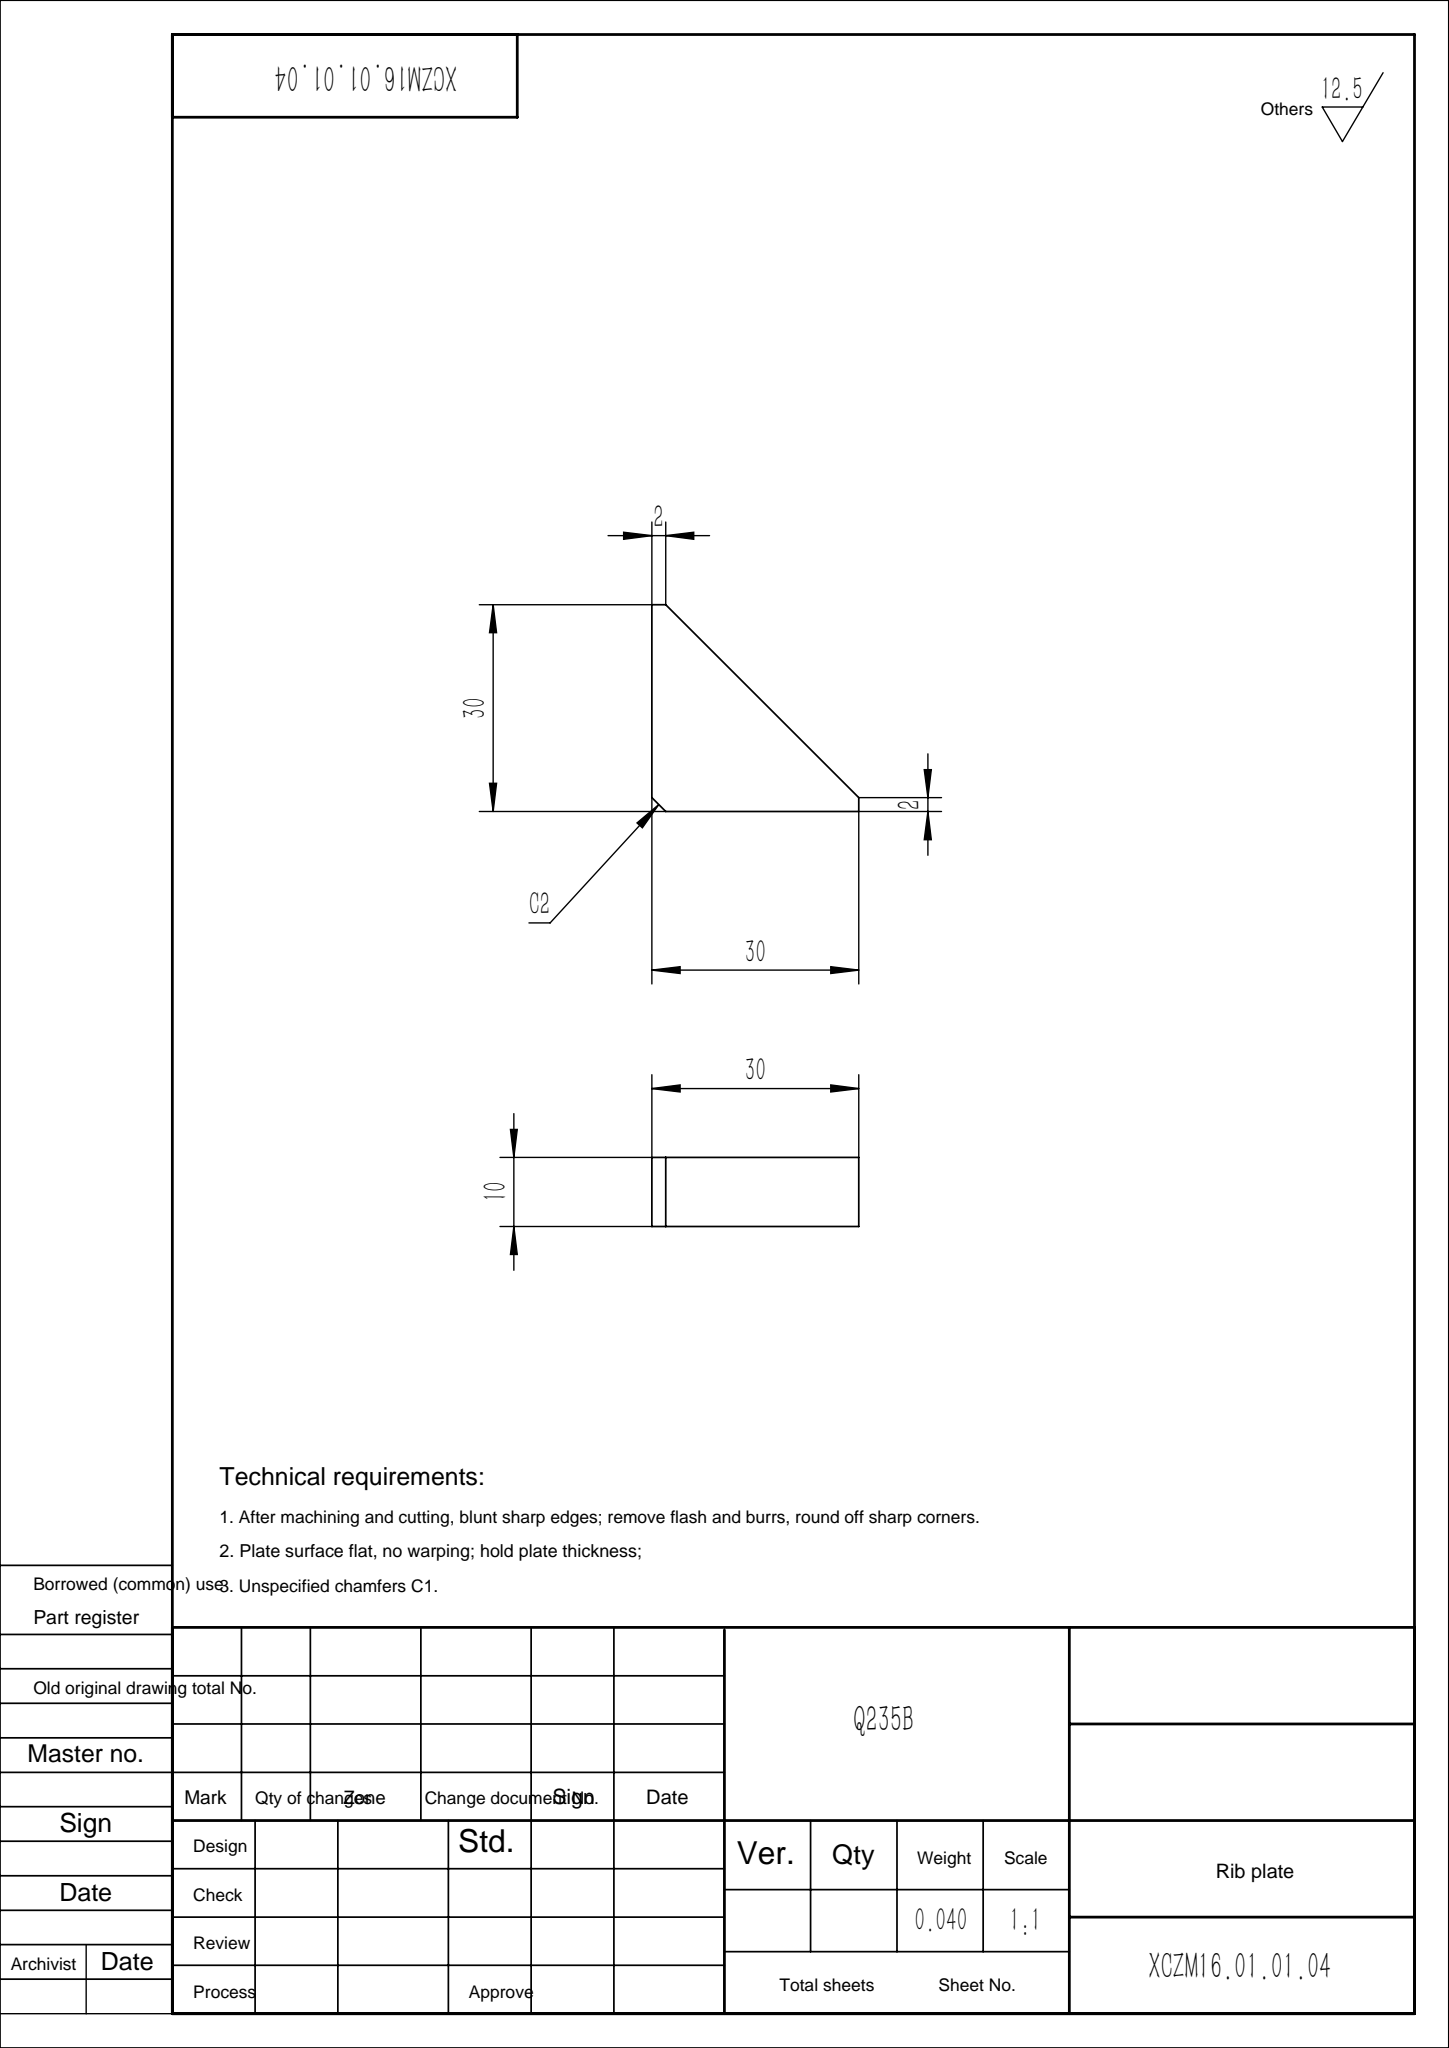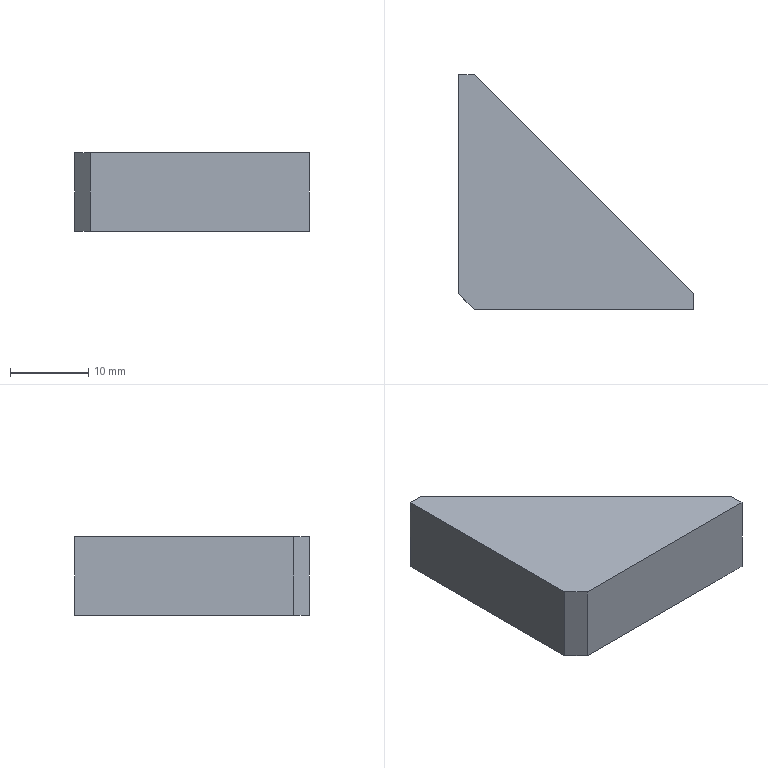Part | SolidWorks | features Chamfer 1, Extrusion 1 | 1 solid | 8 faces | box 30 x 30 x 10 mm | volume 5060 mm3 | plane 8
STEP:
#1=CARTESIAN_POINT('',(2.,30.,0.));
#2=VERTEX_POINT('',#1);
#3=CARTESIAN_POINT('',(0.,30.,0.));
#4=VERTEX_POINT('',#3);
#5=CARTESIAN_POINT('',(2.,30.,0.));
#6=DIRECTION('',(-1.,0.,0.));
#7=VECTOR('',#6,1000.);
#8=LINE('',#5,#7);
#9=EDGE_CURVE('',#2,#4,#8,.T.);
#10=ORIENTED_EDGE('',*,*,#9,.T.);
#11=CARTESIAN_POINT('',(0.,30.,10.));
#12=VERTEX_POINT('',#11);
#13=CARTESIAN_POINT('',(0.,30.,10.));
#14=DIRECTION('',(0.,0.,-1.));
#15=VECTOR('',#14,1000.);
#16=LINE('',#13,#15);
#17=EDGE_CURVE('',#12,#4,#16,.T.);
#18=ORIENTED_EDGE('',*,*,#17,.F.);
#19=CARTESIAN_POINT('',(2.,30.,10.));
#20=VERTEX_POINT('',#19);
#21=CARTESIAN_POINT('',(2.,30.,10.));
#22=DIRECTION('',(-1.,0.,0.));
#23=VECTOR('',#22,1000.);
#24=LINE('',#21,#23);
#25=EDGE_CURVE('',#20,#12,#24,.T.);
#26=ORIENTED_EDGE('',*,*,#25,.F.);
#27=CARTESIAN_POINT('',(2.,30.,10.));
#28=DIRECTION('',(0.,0.,-1.));
#29=VECTOR('',#28,1000.);
#30=LINE('',#27,#29);
#31=EDGE_CURVE('',#20,#2,#30,.T.);
#32=ORIENTED_EDGE('',*,*,#31,.T.);
#33=EDGE_LOOP('',(#10,#18,#26,#32));
#34=FACE_OUTER_BOUND('',#33,.T.);
#35=CARTESIAN_POINT('',(2.,30.,10.));
#36=DIRECTION('',(0.,-1.,0.));
#37=DIRECTION('',(0.,0.,-1.));
#38=AXIS2_PLACEMENT_3D('',#35,#36,#37);
#39=PLANE('',#38);
#40=ADVANCED_FACE('',(#34),#39,.F.);
#41=CARTESIAN_POINT('',(0.,2.,0.));
#42=VERTEX_POINT('',#41);
#43=CARTESIAN_POINT('',(0.,30.,0.));
#44=DIRECTION('',(0.,-1.,0.));
#45=VECTOR('',#44,1000.);
#46=LINE('',#43,#45);
#47=EDGE_CURVE('',#4,#42,#46,.T.);
#48=ORIENTED_EDGE('',*,*,#47,.T.);
#49=CARTESIAN_POINT('',(0.,2.,10.));
#50=VERTEX_POINT('',#49);
#51=CARTESIAN_POINT('',(0.,2.,10.));
#52=DIRECTION('',(0.,0.,1.));
#53=VECTOR('',#52,1000.);
#54=LINE('',#51,#53);
#55=EDGE_CURVE('',#42,#50,#54,.T.);
#56=ORIENTED_EDGE('',*,*,#55,.T.);
#57=CARTESIAN_POINT('',(0.,30.,10.));
#58=DIRECTION('',(0.,-1.,0.));
#59=VECTOR('',#58,1000.);
#60=LINE('',#57,#59);
#61=EDGE_CURVE('',#12,#50,#60,.T.);
#62=ORIENTED_EDGE('',*,*,#61,.F.);
#63=ORIENTED_EDGE('',*,*,#17,.T.);
#64=EDGE_LOOP('',(#48,#56,#62,#63));
#65=FACE_OUTER_BOUND('',#64,.T.);
#66=CARTESIAN_POINT('',(0.,30.,10.));
#67=DIRECTION('',(1.,0.,0.));
#68=DIRECTION('',(0.,1.,0.));
#69=AXIS2_PLACEMENT_3D('',#66,#67,#68);
#70=PLANE('',#69);
#71=ADVANCED_FACE('',(#65),#70,.F.);
#72=CARTESIAN_POINT('',(2.,0.,10.));
#73=VERTEX_POINT('',#72);
#74=CARTESIAN_POINT('',(30.,0.,10.));
#75=VERTEX_POINT('',#74);
#76=CARTESIAN_POINT('',(0.,0.,10.));
#77=DIRECTION('',(1.,0.,0.));
#78=VECTOR('',#77,1000.);
#79=LINE('',#76,#78);
#80=EDGE_CURVE('',#73,#75,#79,.T.);
#81=ORIENTED_EDGE('',*,*,#80,.F.);
#82=CARTESIAN_POINT('',(2.,0.,0.));
#83=VERTEX_POINT('',#82);
#84=CARTESIAN_POINT('',(2.,0.,10.));
#85=DIRECTION('',(0.,0.,-1.));
#86=VECTOR('',#85,1000.);
#87=LINE('',#84,#86);
#88=EDGE_CURVE('',#73,#83,#87,.T.);
#89=ORIENTED_EDGE('',*,*,#88,.T.);
#90=CARTESIAN_POINT('',(30.,0.,0.));
#91=VERTEX_POINT('',#90);
#92=CARTESIAN_POINT('',(0.,0.,0.));
#93=DIRECTION('',(1.,0.,0.));
#94=VECTOR('',#93,1000.);
#95=LINE('',#92,#94);
#96=EDGE_CURVE('',#83,#91,#95,.T.);
#97=ORIENTED_EDGE('',*,*,#96,.T.);
#98=CARTESIAN_POINT('',(30.,0.,10.));
#99=DIRECTION('',(0.,0.,-1.));
#100=VECTOR('',#99,1000.);
#101=LINE('',#98,#100);
#102=EDGE_CURVE('',#75,#91,#101,.T.);
#103=ORIENTED_EDGE('',*,*,#102,.F.);
#104=EDGE_LOOP('',(#81,#89,#97,#103));
#105=FACE_OUTER_BOUND('',#104,.T.);
#106=CARTESIAN_POINT('',(0.,0.,10.));
#107=DIRECTION('',(0.,1.,0.));
#108=DIRECTION('',(0.,0.,1.));
#109=AXIS2_PLACEMENT_3D('',#106,#107,#108);
#110=PLANE('',#109);
#111=ADVANCED_FACE('',(#105),#110,.F.);
#112=CARTESIAN_POINT('',(30.,2.,0.));
#113=VERTEX_POINT('',#112);
#114=CARTESIAN_POINT('',(30.,0.,0.));
#115=DIRECTION('',(0.,1.,0.));
#116=VECTOR('',#115,1000.);
#117=LINE('',#114,#116);
#118=EDGE_CURVE('',#91,#113,#117,.T.);
#119=ORIENTED_EDGE('',*,*,#118,.T.);
#120=CARTESIAN_POINT('',(30.,2.,10.));
#121=VERTEX_POINT('',#120);
#122=CARTESIAN_POINT('',(30.,2.,10.));
#123=DIRECTION('',(0.,0.,-1.));
#124=VECTOR('',#123,1000.);
#125=LINE('',#122,#124);
#126=EDGE_CURVE('',#121,#113,#125,.T.);
#127=ORIENTED_EDGE('',*,*,#126,.F.);
#128=CARTESIAN_POINT('',(30.,0.,10.));
#129=DIRECTION('',(0.,1.,0.));
#130=VECTOR('',#129,1000.);
#131=LINE('',#128,#130);
#132=EDGE_CURVE('',#75,#121,#131,.T.);
#133=ORIENTED_EDGE('',*,*,#132,.F.);
#134=ORIENTED_EDGE('',*,*,#102,.T.);
#135=EDGE_LOOP('',(#119,#127,#133,#134));
#136=FACE_OUTER_BOUND('',#135,.T.);
#137=CARTESIAN_POINT('',(30.,0.,10.));
#138=DIRECTION('',(-1.,0.,0.));
#139=DIRECTION('',(0.,0.,1.));
#140=AXIS2_PLACEMENT_3D('',#137,#138,#139);
#141=PLANE('',#140);
#142=ADVANCED_FACE('',(#136),#141,.F.);
#143=CARTESIAN_POINT('',(30.,2.,0.));
#144=DIRECTION('',(-0.7071,0.7071,0.));
#145=VECTOR('',#144,1000.);
#146=LINE('',#143,#145);
#147=EDGE_CURVE('',#113,#2,#146,.T.);
#148=ORIENTED_EDGE('',*,*,#147,.T.);
#149=ORIENTED_EDGE('',*,*,#31,.F.);
#150=CARTESIAN_POINT('',(30.,2.,10.));
#151=DIRECTION('',(-0.7071,0.7071,0.));
#152=VECTOR('',#151,1000.);
#153=LINE('',#150,#152);
#154=EDGE_CURVE('',#121,#20,#153,.T.);
#155=ORIENTED_EDGE('',*,*,#154,.F.);
#156=ORIENTED_EDGE('',*,*,#126,.T.);
#157=EDGE_LOOP('',(#148,#149,#155,#156));
#158=FACE_OUTER_BOUND('',#157,.T.);
#159=CARTESIAN_POINT('',(30.,2.,10.));
#160=DIRECTION('',(-0.7071,-0.7071,0.));
#161=DIRECTION('',(0.7071,-0.7071,0.));
#162=AXIS2_PLACEMENT_3D('',#159,#160,#161);
#163=PLANE('',#162);
#164=ADVANCED_FACE('',(#158),#163,.F.);
#165=ORIENTED_EDGE('',*,*,#61,.T.);
#166=CARTESIAN_POINT('',(1.,1.,10.));
#167=DIRECTION('',(0.7071,-0.7071,0.));
#168=VECTOR('',#167,1000.);
#169=LINE('',#166,#168);
#170=EDGE_CURVE('',#50,#73,#169,.T.);
#171=ORIENTED_EDGE('',*,*,#170,.T.);
#172=ORIENTED_EDGE('',*,*,#80,.T.);
#173=ORIENTED_EDGE('',*,*,#132,.T.);
#174=ORIENTED_EDGE('',*,*,#154,.T.);
#175=ORIENTED_EDGE('',*,*,#25,.T.);
#176=EDGE_LOOP('',(#165,#171,#172,#173,#174,#175));
#177=FACE_OUTER_BOUND('',#176,.T.);
#178=CARTESIAN_POINT('',(0.,0.,10.));
#179=DIRECTION('',(0.,0.,1.));
#180=DIRECTION('',(1.,0.,0.));
#181=AXIS2_PLACEMENT_3D('',#178,#179,#180);
#182=PLANE('',#181);
#183=ADVANCED_FACE('',(#177),#182,.T.);
#184=ORIENTED_EDGE('',*,*,#96,.F.);
#185=CARTESIAN_POINT('',(2.,0.,0.));
#186=DIRECTION('',(-0.7071,0.7071,0.));
#187=VECTOR('',#186,1000.);
#188=LINE('',#185,#187);
#189=EDGE_CURVE('',#83,#42,#188,.T.);
#190=ORIENTED_EDGE('',*,*,#189,.T.);
#191=ORIENTED_EDGE('',*,*,#47,.F.);
#192=ORIENTED_EDGE('',*,*,#9,.F.);
#193=ORIENTED_EDGE('',*,*,#147,.F.);
#194=ORIENTED_EDGE('',*,*,#118,.F.);
#195=EDGE_LOOP('',(#184,#190,#191,#192,#193,#194));
#196=FACE_OUTER_BOUND('',#195,.T.);
#197=CARTESIAN_POINT('',(0.,0.,0.));
#198=DIRECTION('',(0.,0.,1.));
#199=DIRECTION('',(1.,0.,0.));
#200=AXIS2_PLACEMENT_3D('',#197,#198,#199);
#201=PLANE('',#200);
#202=ADVANCED_FACE('',(#196),#201,.F.);
#203=ORIENTED_EDGE('',*,*,#170,.F.);
#204=ORIENTED_EDGE('',*,*,#55,.F.);
#205=ORIENTED_EDGE('',*,*,#189,.F.);
#206=ORIENTED_EDGE('',*,*,#88,.F.);
#207=EDGE_LOOP('',(#203,#204,#205,#206));
#208=FACE_OUTER_BOUND('',#207,.T.);
#209=CARTESIAN_POINT('',(2.,0.,10.));
#210=DIRECTION('',(0.7071,0.7071,0.));
#211=DIRECTION('',(0.,0.,-1.));
#212=AXIS2_PLACEMENT_3D('',#209,#210,#211);
#213=PLANE('',#212);
#214=ADVANCED_FACE('',(#208),#213,.F.);
#215=CLOSED_SHELL('',(#40,#71,#111,#142,#164,#183,#202,#214));
#216=MANIFOLD_SOLID_BREP('',#215);
#217=CARTESIAN_POINT('',(0.,0.,0.));
#218=DIRECTION('',(0.,0.,1.));
#219=DIRECTION('',(1.,0.,0.));
#220=AXIS2_PLACEMENT_3D('',#217,#218,#219);
#221=(LENGTH_UNIT()NAMED_UNIT(*)SI_UNIT(.MILLI.,.METRE.));
#222=UNCERTAINTY_MEASURE_WITH_UNIT(LENGTH_MEASURE(0.00001),#221,'','');
#223=(NAMED_UNIT(*)PLANE_ANGLE_UNIT()SI_UNIT($,.RADIAN.));
#224=(NAMED_UNIT(*)SI_UNIT($,.STERADIAN.)SOLID_ANGLE_UNIT());
#225=(GEOMETRIC_REPRESENTATION_CONTEXT(3)GLOBAL_UNCERTAINTY_ASSIGNED_CONTEXT((#222))GLOBAL_UNIT_ASSIGNED_CONTEXT((#221,#223,#224))REPRESENTATION_CONTEXT('',''));
#226=ADVANCED_BREP_SHAPE_REPRESENTATION('',(#216,#220),#225);